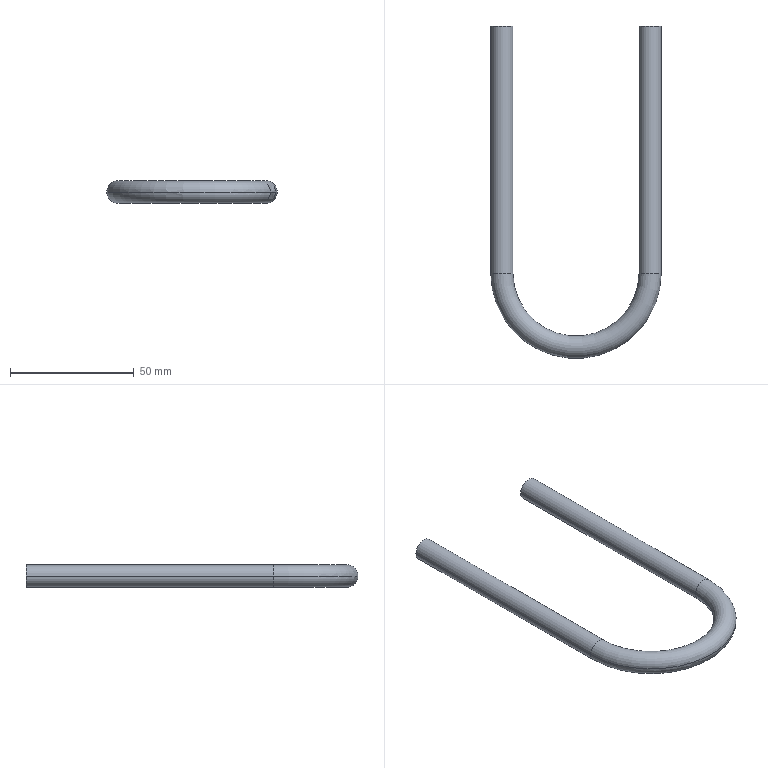Part | SolidWorks | features Sweep 1 | 1 solid | 8 faces | box 69 x 134.5 x 9 mm | volume 18719 mm3 | cylinder 4 | torus 2 | plane 2 | commonest cylinder face diameters 9 x4
STEP:
#1=CARTESIAN_POINT('',(-4.5,-100.,0.));
#2=VERTEX_POINT('',#1);
#3=CARTESIAN_POINT('',(4.5,-100.,0.));
#4=VERTEX_POINT('',#3);
#5=CARTESIAN_POINT('',(0.,-100.,0.));
#6=DIRECTION('',(0.,1.,0.));
#7=DIRECTION('',(0.,0.,1.));
#8=AXIS2_PLACEMENT_3D('',#5,#6,#7);
#9=CIRCLE('',#8,4.5);
#10=EDGE_CURVE('',#2,#4,#9,.T.);
#11=ORIENTED_EDGE('',*,*,#10,.F.);
#12=CARTESIAN_POINT('',(64.5,-100.,0.));
#13=VERTEX_POINT('',#12);
#14=CARTESIAN_POINT('',(30.,-100.,0.));
#15=DIRECTION('',(0.,0.,1.));
#16=DIRECTION('',(1.,0.,0.));
#17=AXIS2_PLACEMENT_3D('',#14,#15,#16);
#18=CIRCLE('',#17,34.5);
#19=EDGE_CURVE('',#2,#13,#18,.T.);
#20=ORIENTED_EDGE('',*,*,#19,.T.);
#21=CARTESIAN_POINT('',(55.5,-100.,0.));
#22=VERTEX_POINT('',#21);
#23=CARTESIAN_POINT('',(60.,-100.,0.));
#24=DIRECTION('',(0.,-1.,0.));
#25=DIRECTION('',(0.,0.,1.));
#26=AXIS2_PLACEMENT_3D('',#23,#24,#25);
#27=CIRCLE('',#26,4.5);
#28=EDGE_CURVE('',#13,#22,#27,.T.);
#29=ORIENTED_EDGE('',*,*,#28,.T.);
#30=CARTESIAN_POINT('',(30.,-100.,0.));
#31=DIRECTION('',(0.,0.,1.));
#32=DIRECTION('',(1.,0.,0.));
#33=AXIS2_PLACEMENT_3D('',#30,#31,#32);
#34=CIRCLE('',#33,25.5);
#35=EDGE_CURVE('',#4,#22,#34,.T.);
#36=ORIENTED_EDGE('',*,*,#35,.F.);
#37=EDGE_LOOP('',(#11,#20,#29,#36));
#38=FACE_OUTER_BOUND('',#37,.T.);
#39=CARTESIAN_POINT('',(30.,-100.,0.));
#40=DIRECTION('',(0.,0.,1.));
#41=DIRECTION('',(1.,0.,0.));
#42=AXIS2_PLACEMENT_3D('',#39,#40,#41);
#43=TOROIDAL_SURFACE('',#42,30.,4.5);
#44=ADVANCED_FACE('',(#38),#43,.T.);
#45=ORIENTED_EDGE('',*,*,#10,.T.);
#46=CARTESIAN_POINT('',(4.5,0.,0.));
#47=VERTEX_POINT('',#46);
#48=CARTESIAN_POINT('',(4.5,-100.,0.));
#49=DIRECTION('',(0.,1.,0.));
#50=VECTOR('',#49,1000.);
#51=LINE('',#48,#50);
#52=EDGE_CURVE('',#4,#47,#51,.T.);
#53=ORIENTED_EDGE('',*,*,#52,.T.);
#54=CARTESIAN_POINT('',(-4.5,0.,0.));
#55=VERTEX_POINT('',#54);
#56=CARTESIAN_POINT('',(0.,0.,0.));
#57=DIRECTION('',(0.,1.,0.));
#58=DIRECTION('',(0.,0.,1.));
#59=AXIS2_PLACEMENT_3D('',#56,#57,#58);
#60=CIRCLE('',#59,4.5);
#61=EDGE_CURVE('',#55,#47,#60,.T.);
#62=ORIENTED_EDGE('',*,*,#61,.F.);
#63=CARTESIAN_POINT('',(-4.5,-100.,0.));
#64=DIRECTION('',(0.,1.,0.));
#65=VECTOR('',#64,1000.);
#66=LINE('',#63,#65);
#67=EDGE_CURVE('',#2,#55,#66,.T.);
#68=ORIENTED_EDGE('',*,*,#67,.F.);
#69=EDGE_LOOP('',(#45,#53,#62,#68));
#70=FACE_OUTER_BOUND('',#69,.T.);
#71=CARTESIAN_POINT('',(0.,-100.,0.));
#72=DIRECTION('',(0.,1.,0.));
#73=DIRECTION('',(-1.,0.,0.));
#74=AXIS2_PLACEMENT_3D('',#71,#72,#73);
#75=CYLINDRICAL_SURFACE('',#74,4.5);
#76=ADVANCED_FACE('',(#70),#75,.T.);
#77=ORIENTED_EDGE('',*,*,#28,.F.);
#78=CARTESIAN_POINT('',(64.5,0.,0.));
#79=VERTEX_POINT('',#78);
#80=CARTESIAN_POINT('',(64.5,-100.,0.));
#81=DIRECTION('',(0.,1.,0.));
#82=VECTOR('',#81,1000.);
#83=LINE('',#80,#82);
#84=EDGE_CURVE('',#13,#79,#83,.T.);
#85=ORIENTED_EDGE('',*,*,#84,.T.);
#86=CARTESIAN_POINT('',(55.5,0.,0.));
#87=VERTEX_POINT('',#86);
#88=CARTESIAN_POINT('',(60.,0.,0.));
#89=DIRECTION('',(0.,-1.,0.));
#90=DIRECTION('',(0.,0.,1.));
#91=AXIS2_PLACEMENT_3D('',#88,#89,#90);
#92=CIRCLE('',#91,4.5);
#93=EDGE_CURVE('',#79,#87,#92,.T.);
#94=ORIENTED_EDGE('',*,*,#93,.T.);
#95=CARTESIAN_POINT('',(55.5,-100.,0.));
#96=DIRECTION('',(0.,1.,0.));
#97=VECTOR('',#96,1000.);
#98=LINE('',#95,#97);
#99=EDGE_CURVE('',#22,#87,#98,.T.);
#100=ORIENTED_EDGE('',*,*,#99,.F.);
#101=EDGE_LOOP('',(#77,#85,#94,#100));
#102=FACE_OUTER_BOUND('',#101,.T.);
#103=CARTESIAN_POINT('',(60.,-100.,0.));
#104=DIRECTION('',(0.,1.,0.));
#105=DIRECTION('',(-1.,0.,0.));
#106=AXIS2_PLACEMENT_3D('',#103,#104,#105);
#107=CYLINDRICAL_SURFACE('',#106,4.5);
#108=ADVANCED_FACE('',(#102),#107,.T.);
#109=ORIENTED_EDGE('',*,*,#84,.F.);
#110=CARTESIAN_POINT('',(60.,-100.,0.));
#111=DIRECTION('',(0.,-1.,0.));
#112=DIRECTION('',(0.,0.,1.));
#113=AXIS2_PLACEMENT_3D('',#110,#111,#112);
#114=CIRCLE('',#113,4.5);
#115=EDGE_CURVE('',#22,#13,#114,.T.);
#116=ORIENTED_EDGE('',*,*,#115,.F.);
#117=ORIENTED_EDGE('',*,*,#99,.T.);
#118=CARTESIAN_POINT('',(60.,0.,0.));
#119=DIRECTION('',(0.,-1.,0.));
#120=DIRECTION('',(0.,0.,1.));
#121=AXIS2_PLACEMENT_3D('',#118,#119,#120);
#122=CIRCLE('',#121,4.5);
#123=EDGE_CURVE('',#87,#79,#122,.T.);
#124=ORIENTED_EDGE('',*,*,#123,.T.);
#125=EDGE_LOOP('',(#109,#116,#117,#124));
#126=FACE_OUTER_BOUND('',#125,.T.);
#127=CARTESIAN_POINT('',(60.,-100.,0.));
#128=DIRECTION('',(0.,1.,0.));
#129=DIRECTION('',(-1.,0.,0.));
#130=AXIS2_PLACEMENT_3D('',#127,#128,#129);
#131=CYLINDRICAL_SURFACE('',#130,4.5);
#132=ADVANCED_FACE('',(#126),#131,.T.);
#133=ORIENTED_EDGE('',*,*,#19,.F.);
#134=CARTESIAN_POINT('',(0.,-100.,0.));
#135=DIRECTION('',(0.,1.,0.));
#136=DIRECTION('',(0.,0.,1.));
#137=AXIS2_PLACEMENT_3D('',#134,#135,#136);
#138=CIRCLE('',#137,4.5);
#139=EDGE_CURVE('',#4,#2,#138,.T.);
#140=ORIENTED_EDGE('',*,*,#139,.F.);
#141=ORIENTED_EDGE('',*,*,#35,.T.);
#142=ORIENTED_EDGE('',*,*,#115,.T.);
#143=EDGE_LOOP('',(#133,#140,#141,#142));
#144=FACE_OUTER_BOUND('',#143,.T.);
#145=CARTESIAN_POINT('',(30.,-100.,0.));
#146=DIRECTION('',(0.,0.,1.));
#147=DIRECTION('',(1.,0.,0.));
#148=AXIS2_PLACEMENT_3D('',#145,#146,#147);
#149=TOROIDAL_SURFACE('',#148,30.,4.5);
#150=ADVANCED_FACE('',(#144),#149,.T.);
#151=ORIENTED_EDGE('',*,*,#52,.F.);
#152=ORIENTED_EDGE('',*,*,#139,.T.);
#153=ORIENTED_EDGE('',*,*,#67,.T.);
#154=CARTESIAN_POINT('',(0.,0.,0.));
#155=DIRECTION('',(0.,1.,0.));
#156=DIRECTION('',(0.,0.,1.));
#157=AXIS2_PLACEMENT_3D('',#154,#155,#156);
#158=CIRCLE('',#157,4.5);
#159=EDGE_CURVE('',#47,#55,#158,.T.);
#160=ORIENTED_EDGE('',*,*,#159,.F.);
#161=EDGE_LOOP('',(#151,#152,#153,#160));
#162=FACE_OUTER_BOUND('',#161,.T.);
#163=CARTESIAN_POINT('',(0.,-100.,0.));
#164=DIRECTION('',(0.,1.,0.));
#165=DIRECTION('',(-1.,0.,0.));
#166=AXIS2_PLACEMENT_3D('',#163,#164,#165);
#167=CYLINDRICAL_SURFACE('',#166,4.5);
#168=ADVANCED_FACE('',(#162),#167,.T.);
#169=ORIENTED_EDGE('',*,*,#123,.F.);
#170=ORIENTED_EDGE('',*,*,#93,.F.);
#171=EDGE_LOOP('',(#169,#170));
#172=FACE_OUTER_BOUND('',#171,.T.);
#173=CARTESIAN_POINT('',(60.,0.,0.));
#174=DIRECTION('',(0.,-1.,0.));
#175=DIRECTION('',(0.,0.,1.));
#176=AXIS2_PLACEMENT_3D('',#173,#174,#175);
#177=PLANE('',#176);
#178=ADVANCED_FACE('',(#172),#177,.F.);
#179=ORIENTED_EDGE('',*,*,#61,.T.);
#180=ORIENTED_EDGE('',*,*,#159,.T.);
#181=EDGE_LOOP('',(#179,#180));
#182=FACE_OUTER_BOUND('',#181,.T.);
#183=CARTESIAN_POINT('',(0.,0.,0.));
#184=DIRECTION('',(0.,1.,0.));
#185=DIRECTION('',(0.,0.,1.));
#186=AXIS2_PLACEMENT_3D('',#183,#184,#185);
#187=PLANE('',#186);
#188=ADVANCED_FACE('',(#182),#187,.T.);
#189=CLOSED_SHELL('',(#44,#76,#108,#132,#150,#168,#178,#188));
#190=MANIFOLD_SOLID_BREP('',#189);
#191=CARTESIAN_POINT('',(0.,0.,0.));
#192=DIRECTION('',(0.,0.,1.));
#193=DIRECTION('',(1.,0.,0.));
#194=AXIS2_PLACEMENT_3D('',#191,#192,#193);
#195=(LENGTH_UNIT()NAMED_UNIT(*)SI_UNIT(.MILLI.,.METRE.));
#196=UNCERTAINTY_MEASURE_WITH_UNIT(LENGTH_MEASURE(0.00001),#195,'','');
#197=(NAMED_UNIT(*)PLANE_ANGLE_UNIT()SI_UNIT($,.RADIAN.));
#198=(NAMED_UNIT(*)SI_UNIT($,.STERADIAN.)SOLID_ANGLE_UNIT());
#199=(GEOMETRIC_REPRESENTATION_CONTEXT(3)GLOBAL_UNCERTAINTY_ASSIGNED_CONTEXT((#196))GLOBAL_UNIT_ASSIGNED_CONTEXT((#195,#197,#198))REPRESENTATION_CONTEXT('',''));
#200=ADVANCED_BREP_SHAPE_REPRESENTATION('',(#190,#194),#199);